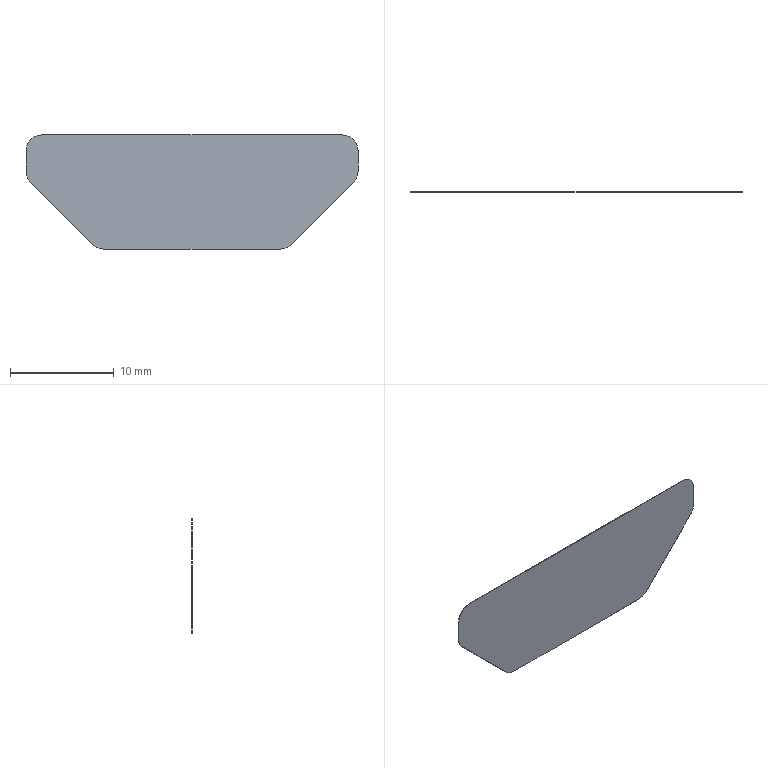Part | NX | features BREP 1 | 1 solid | 14 faces | box 32 x 0.05 x 11 mm | volume 15.176 mm3 | plane 8 | cylinder 6 | commonest cylinder face diameters 3 x6
STEP:
#1=CARTESIAN_POINT('',(0.,0.,7.5));
#2=VERTEX_POINT('',#1);
#3=CARTESIAN_POINT('',(0.,0.05,7.5));
#4=VERTEX_POINT('',#3);
#5=CARTESIAN_POINT('',(0.,0.,7.5));
#6=DIRECTION('',(0.,1.,0.));
#7=VECTOR('',#6,1000.);
#8=LINE('',#5,#7);
#9=EDGE_CURVE('',#2,#4,#8,.T.);
#10=ORIENTED_EDGE('',*,*,#9,.F.);
#11=CARTESIAN_POINT('',(0.,0.,9.5));
#12=VERTEX_POINT('',#11);
#13=CARTESIAN_POINT('',(0.,0.,7.5));
#14=DIRECTION('',(0.,0.,1.));
#15=VECTOR('',#14,1000.);
#16=LINE('',#13,#15);
#17=EDGE_CURVE('',#2,#12,#16,.T.);
#18=ORIENTED_EDGE('',*,*,#17,.T.);
#19=CARTESIAN_POINT('',(0.,0.05,9.5));
#20=VERTEX_POINT('',#19);
#21=CARTESIAN_POINT('',(0.,0.,9.5));
#22=DIRECTION('',(0.,1.,0.));
#23=VECTOR('',#22,1000.);
#24=LINE('',#21,#23);
#25=EDGE_CURVE('',#12,#20,#24,.T.);
#26=ORIENTED_EDGE('',*,*,#25,.T.);
#27=CARTESIAN_POINT('',(0.,0.05,7.5));
#28=DIRECTION('',(0.,0.,1.));
#29=VECTOR('',#28,1000.);
#30=LINE('',#27,#29);
#31=EDGE_CURVE('',#4,#20,#30,.T.);
#32=ORIENTED_EDGE('',*,*,#31,.F.);
#33=EDGE_LOOP('',(#10,#18,#26,#32));
#34=FACE_BOUND('',#33,.T.);
#35=CARTESIAN_POINT('',(0.,0.,7.5));
#36=DIRECTION('',(-1.,0.,0.));
#37=DIRECTION('',(0.,0.,-1.));
#38=AXIS2_PLACEMENT_3D('',#35,#36,#37);
#39=PLANE('',#38);
#40=ADVANCED_FACE('',(#34),#39,.T.);
#41=ORIENTED_EDGE('',*,*,#25,.F.);
#42=CARTESIAN_POINT('',(1.5,0.,11.));
#43=VERTEX_POINT('',#42);
#44=CARTESIAN_POINT('',(1.5,0.,9.5));
#45=DIRECTION('',(0.,1.,0.));
#46=DIRECTION('',(-1.,0.,0.));
#47=AXIS2_PLACEMENT_3D('',#44,#45,#46);
#48=CIRCLE('',#47,1.5);
#49=EDGE_CURVE('',#12,#43,#48,.T.);
#50=ORIENTED_EDGE('',*,*,#49,.T.);
#51=CARTESIAN_POINT('',(1.5,0.05,11.));
#52=VERTEX_POINT('',#51);
#53=CARTESIAN_POINT('',(1.5,0.,11.));
#54=DIRECTION('',(0.,1.,0.));
#55=VECTOR('',#54,1000.);
#56=LINE('',#53,#55);
#57=EDGE_CURVE('',#43,#52,#56,.T.);
#58=ORIENTED_EDGE('',*,*,#57,.T.);
#59=CARTESIAN_POINT('',(1.5,0.05,9.5));
#60=DIRECTION('',(0.,1.,0.));
#61=DIRECTION('',(-1.,0.,0.));
#62=AXIS2_PLACEMENT_3D('',#59,#60,#61);
#63=CIRCLE('',#62,1.5);
#64=EDGE_CURVE('',#20,#52,#63,.T.);
#65=ORIENTED_EDGE('',*,*,#64,.F.);
#66=EDGE_LOOP('',(#41,#50,#58,#65));
#67=FACE_BOUND('',#66,.T.);
#68=CARTESIAN_POINT('',(1.5,0.,9.5));
#69=DIRECTION('',(0.,1.,0.));
#70=DIRECTION('',(-0.7071,0.,0.7071));
#71=AXIS2_PLACEMENT_3D('',#68,#69,#70);
#72=CYLINDRICAL_SURFACE('',#71,1.5);
#73=ADVANCED_FACE('',(#67),#72,.T.);
#74=ORIENTED_EDGE('',*,*,#57,.F.);
#75=CARTESIAN_POINT('',(30.5,0.,11.));
#76=VERTEX_POINT('',#75);
#77=CARTESIAN_POINT('',(1.5,0.,11.));
#78=DIRECTION('',(1.,0.,0.));
#79=VECTOR('',#78,1000.);
#80=LINE('',#77,#79);
#81=EDGE_CURVE('',#43,#76,#80,.T.);
#82=ORIENTED_EDGE('',*,*,#81,.T.);
#83=CARTESIAN_POINT('',(30.5,0.05,11.));
#84=VERTEX_POINT('',#83);
#85=CARTESIAN_POINT('',(30.5,0.,11.));
#86=DIRECTION('',(0.,1.,0.));
#87=VECTOR('',#86,1000.);
#88=LINE('',#85,#87);
#89=EDGE_CURVE('',#76,#84,#88,.T.);
#90=ORIENTED_EDGE('',*,*,#89,.T.);
#91=CARTESIAN_POINT('',(1.5,0.05,11.));
#92=DIRECTION('',(1.,0.,0.));
#93=VECTOR('',#92,1000.);
#94=LINE('',#91,#93);
#95=EDGE_CURVE('',#52,#84,#94,.T.);
#96=ORIENTED_EDGE('',*,*,#95,.F.);
#97=EDGE_LOOP('',(#74,#82,#90,#96));
#98=FACE_BOUND('',#97,.T.);
#99=CARTESIAN_POINT('',(1.5,0.,11.));
#100=DIRECTION('',(0.,0.,1.));
#101=DIRECTION('',(-1.,0.,0.));
#102=AXIS2_PLACEMENT_3D('',#99,#100,#101);
#103=PLANE('',#102);
#104=ADVANCED_FACE('',(#98),#103,.T.);
#105=ORIENTED_EDGE('',*,*,#89,.F.);
#106=CARTESIAN_POINT('',(32.,0.,9.5));
#107=VERTEX_POINT('',#106);
#108=CARTESIAN_POINT('',(30.5,0.,9.5));
#109=DIRECTION('',(0.,1.,0.));
#110=DIRECTION('',(0.,0.,1.));
#111=AXIS2_PLACEMENT_3D('',#108,#109,#110);
#112=CIRCLE('',#111,1.5);
#113=EDGE_CURVE('',#76,#107,#112,.T.);
#114=ORIENTED_EDGE('',*,*,#113,.T.);
#115=CARTESIAN_POINT('',(32.,0.05,9.5));
#116=VERTEX_POINT('',#115);
#117=CARTESIAN_POINT('',(32.,0.,9.5));
#118=DIRECTION('',(0.,1.,0.));
#119=VECTOR('',#118,1000.);
#120=LINE('',#117,#119);
#121=EDGE_CURVE('',#107,#116,#120,.T.);
#122=ORIENTED_EDGE('',*,*,#121,.T.);
#123=CARTESIAN_POINT('',(30.5,0.05,9.5));
#124=DIRECTION('',(0.,1.,0.));
#125=DIRECTION('',(0.,0.,1.));
#126=AXIS2_PLACEMENT_3D('',#123,#124,#125);
#127=CIRCLE('',#126,1.5);
#128=EDGE_CURVE('',#84,#116,#127,.T.);
#129=ORIENTED_EDGE('',*,*,#128,.F.);
#130=EDGE_LOOP('',(#105,#114,#122,#129));
#131=FACE_BOUND('',#130,.T.);
#132=CARTESIAN_POINT('',(30.5,0.,9.5));
#133=DIRECTION('',(0.,1.,0.));
#134=DIRECTION('',(0.7071,0.,0.7071));
#135=AXIS2_PLACEMENT_3D('',#132,#133,#134);
#136=CYLINDRICAL_SURFACE('',#135,1.5);
#137=ADVANCED_FACE('',(#131),#136,.T.);
#138=ORIENTED_EDGE('',*,*,#121,.F.);
#139=CARTESIAN_POINT('',(32.,0.,7.5));
#140=VERTEX_POINT('',#139);
#141=CARTESIAN_POINT('',(32.,0.,9.5));
#142=DIRECTION('',(0.,0.,-1.));
#143=VECTOR('',#142,1000.);
#144=LINE('',#141,#143);
#145=EDGE_CURVE('',#107,#140,#144,.T.);
#146=ORIENTED_EDGE('',*,*,#145,.T.);
#147=CARTESIAN_POINT('',(32.,0.05,7.5));
#148=VERTEX_POINT('',#147);
#149=CARTESIAN_POINT('',(32.,0.,7.5));
#150=DIRECTION('',(0.,1.,0.));
#151=VECTOR('',#150,1000.);
#152=LINE('',#149,#151);
#153=EDGE_CURVE('',#140,#148,#152,.T.);
#154=ORIENTED_EDGE('',*,*,#153,.T.);
#155=CARTESIAN_POINT('',(32.,0.05,9.5));
#156=DIRECTION('',(0.,0.,-1.));
#157=VECTOR('',#156,1000.);
#158=LINE('',#155,#157);
#159=EDGE_CURVE('',#116,#148,#158,.T.);
#160=ORIENTED_EDGE('',*,*,#159,.F.);
#161=EDGE_LOOP('',(#138,#146,#154,#160));
#162=FACE_BOUND('',#161,.T.);
#163=CARTESIAN_POINT('',(32.,0.,9.5));
#164=DIRECTION('',(1.,0.,0.));
#165=DIRECTION('',(0.,-1.,0.));
#166=AXIS2_PLACEMENT_3D('',#163,#164,#165);
#167=PLANE('',#166);
#168=ADVANCED_FACE('',(#162),#167,.T.);
#169=ORIENTED_EDGE('',*,*,#153,.F.);
#170=CARTESIAN_POINT('',(31.561,0.,6.439));
#171=VERTEX_POINT('',#170);
#172=CARTESIAN_POINT('',(30.5,0.,7.5));
#173=DIRECTION('',(0.,1.,0.));
#174=DIRECTION('',(1.,0.,0.));
#175=AXIS2_PLACEMENT_3D('',#172,#173,#174);
#176=CIRCLE('',#175,1.5);
#177=EDGE_CURVE('',#140,#171,#176,.T.);
#178=ORIENTED_EDGE('',*,*,#177,.T.);
#179=CARTESIAN_POINT('',(31.561,0.05,6.439));
#180=VERTEX_POINT('',#179);
#181=CARTESIAN_POINT('',(31.561,0.,6.439));
#182=DIRECTION('',(0.,1.,0.));
#183=VECTOR('',#182,1000.);
#184=LINE('',#181,#183);
#185=EDGE_CURVE('',#171,#180,#184,.T.);
#186=ORIENTED_EDGE('',*,*,#185,.T.);
#187=CARTESIAN_POINT('',(30.5,0.05,7.5));
#188=DIRECTION('',(0.,1.,0.));
#189=DIRECTION('',(1.,0.,0.));
#190=AXIS2_PLACEMENT_3D('',#187,#188,#189);
#191=CIRCLE('',#190,1.5);
#192=EDGE_CURVE('',#148,#180,#191,.T.);
#193=ORIENTED_EDGE('',*,*,#192,.F.);
#194=EDGE_LOOP('',(#169,#178,#186,#193));
#195=FACE_BOUND('',#194,.T.);
#196=CARTESIAN_POINT('',(30.5,0.,7.5));
#197=DIRECTION('',(0.,1.,0.));
#198=DIRECTION('',(0.9239,0.,-0.3827));
#199=AXIS2_PLACEMENT_3D('',#196,#197,#198);
#200=CYLINDRICAL_SURFACE('',#199,1.5);
#201=ADVANCED_FACE('',(#195),#200,.T.);
#202=ORIENTED_EDGE('',*,*,#185,.F.);
#203=CARTESIAN_POINT('',(25.561,0.,0.4393));
#204=VERTEX_POINT('',#203);
#205=CARTESIAN_POINT('',(31.561,0.,6.439));
#206=DIRECTION('',(-0.7071,0.,-0.7071));
#207=VECTOR('',#206,1000.);
#208=LINE('',#205,#207);
#209=EDGE_CURVE('',#171,#204,#208,.T.);
#210=ORIENTED_EDGE('',*,*,#209,.T.);
#211=CARTESIAN_POINT('',(25.561,0.05,0.4393));
#212=VERTEX_POINT('',#211);
#213=CARTESIAN_POINT('',(25.561,0.,0.4393));
#214=DIRECTION('',(0.,1.,0.));
#215=VECTOR('',#214,1000.);
#216=LINE('',#213,#215);
#217=EDGE_CURVE('',#204,#212,#216,.T.);
#218=ORIENTED_EDGE('',*,*,#217,.T.);
#219=CARTESIAN_POINT('',(31.561,0.05,6.439));
#220=DIRECTION('',(-0.7071,0.,-0.7071));
#221=VECTOR('',#220,1000.);
#222=LINE('',#219,#221);
#223=EDGE_CURVE('',#180,#212,#222,.T.);
#224=ORIENTED_EDGE('',*,*,#223,.F.);
#225=EDGE_LOOP('',(#202,#210,#218,#224));
#226=FACE_BOUND('',#225,.T.);
#227=CARTESIAN_POINT('',(31.561,0.,6.439));
#228=DIRECTION('',(0.7071,0.,-0.7071));
#229=DIRECTION('',(0.,1.,0.));
#230=AXIS2_PLACEMENT_3D('',#227,#228,#229);
#231=PLANE('',#230);
#232=ADVANCED_FACE('',(#226),#231,.T.);
#233=ORIENTED_EDGE('',*,*,#217,.F.);
#234=CARTESIAN_POINT('',(24.5,0.,0.));
#235=VERTEX_POINT('',#234);
#236=CARTESIAN_POINT('',(24.5,0.,1.5));
#237=DIRECTION('',(0.,1.,0.));
#238=DIRECTION('',(0.7071,0.,-0.7071));
#239=AXIS2_PLACEMENT_3D('',#236,#237,#238);
#240=CIRCLE('',#239,1.5);
#241=EDGE_CURVE('',#204,#235,#240,.T.);
#242=ORIENTED_EDGE('',*,*,#241,.T.);
#243=CARTESIAN_POINT('',(24.5,0.05,0.));
#244=VERTEX_POINT('',#243);
#245=CARTESIAN_POINT('',(24.5,0.,0.));
#246=DIRECTION('',(0.,1.,0.));
#247=VECTOR('',#246,1000.);
#248=LINE('',#245,#247);
#249=EDGE_CURVE('',#235,#244,#248,.T.);
#250=ORIENTED_EDGE('',*,*,#249,.T.);
#251=CARTESIAN_POINT('',(24.5,0.05,1.5));
#252=DIRECTION('',(0.,1.,0.));
#253=DIRECTION('',(0.7071,0.,-0.7071));
#254=AXIS2_PLACEMENT_3D('',#251,#252,#253);
#255=CIRCLE('',#254,1.5);
#256=EDGE_CURVE('',#212,#244,#255,.T.);
#257=ORIENTED_EDGE('',*,*,#256,.F.);
#258=EDGE_LOOP('',(#233,#242,#250,#257));
#259=FACE_BOUND('',#258,.T.);
#260=CARTESIAN_POINT('',(24.5,0.,1.5));
#261=DIRECTION('',(0.,1.,0.));
#262=DIRECTION('',(0.3827,0.,-0.9239));
#263=AXIS2_PLACEMENT_3D('',#260,#261,#262);
#264=CYLINDRICAL_SURFACE('',#263,1.5);
#265=ADVANCED_FACE('',(#259),#264,.T.);
#266=ORIENTED_EDGE('',*,*,#249,.F.);
#267=CARTESIAN_POINT('',(7.5,0.,0.));
#268=VERTEX_POINT('',#267);
#269=CARTESIAN_POINT('',(24.5,0.,0.));
#270=DIRECTION('',(-1.,0.,0.));
#271=VECTOR('',#270,1000.);
#272=LINE('',#269,#271);
#273=EDGE_CURVE('',#235,#268,#272,.T.);
#274=ORIENTED_EDGE('',*,*,#273,.T.);
#275=CARTESIAN_POINT('',(7.5,0.05,0.));
#276=VERTEX_POINT('',#275);
#277=CARTESIAN_POINT('',(7.5,0.,0.));
#278=DIRECTION('',(0.,1.,0.));
#279=VECTOR('',#278,1000.);
#280=LINE('',#277,#279);
#281=EDGE_CURVE('',#268,#276,#280,.T.);
#282=ORIENTED_EDGE('',*,*,#281,.T.);
#283=CARTESIAN_POINT('',(24.5,0.05,0.));
#284=DIRECTION('',(-1.,0.,0.));
#285=VECTOR('',#284,1000.);
#286=LINE('',#283,#285);
#287=EDGE_CURVE('',#244,#276,#286,.T.);
#288=ORIENTED_EDGE('',*,*,#287,.F.);
#289=EDGE_LOOP('',(#266,#274,#282,#288));
#290=FACE_BOUND('',#289,.T.);
#291=CARTESIAN_POINT('',(24.5,0.,0.));
#292=DIRECTION('',(0.,0.,-1.));
#293=DIRECTION('',(0.,1.,0.));
#294=AXIS2_PLACEMENT_3D('',#291,#292,#293);
#295=PLANE('',#294);
#296=ADVANCED_FACE('',(#290),#295,.T.);
#297=ORIENTED_EDGE('',*,*,#281,.F.);
#298=CARTESIAN_POINT('',(6.439,0.,0.4393));
#299=VERTEX_POINT('',#298);
#300=CARTESIAN_POINT('',(7.5,0.,1.5));
#301=DIRECTION('',(0.,1.,0.));
#302=DIRECTION('',(0.,0.,-1.));
#303=AXIS2_PLACEMENT_3D('',#300,#301,#302);
#304=CIRCLE('',#303,1.5);
#305=EDGE_CURVE('',#268,#299,#304,.T.);
#306=ORIENTED_EDGE('',*,*,#305,.T.);
#307=CARTESIAN_POINT('',(6.439,0.05,0.4393));
#308=VERTEX_POINT('',#307);
#309=CARTESIAN_POINT('',(6.439,0.,0.4393));
#310=DIRECTION('',(0.,1.,0.));
#311=VECTOR('',#310,1000.);
#312=LINE('',#309,#311);
#313=EDGE_CURVE('',#299,#308,#312,.T.);
#314=ORIENTED_EDGE('',*,*,#313,.T.);
#315=CARTESIAN_POINT('',(7.5,0.05,1.5));
#316=DIRECTION('',(0.,1.,0.));
#317=DIRECTION('',(0.,0.,-1.));
#318=AXIS2_PLACEMENT_3D('',#315,#316,#317);
#319=CIRCLE('',#318,1.5);
#320=EDGE_CURVE('',#276,#308,#319,.T.);
#321=ORIENTED_EDGE('',*,*,#320,.F.);
#322=EDGE_LOOP('',(#297,#306,#314,#321));
#323=FACE_BOUND('',#322,.T.);
#324=CARTESIAN_POINT('',(7.5,0.,1.5));
#325=DIRECTION('',(0.,1.,0.));
#326=DIRECTION('',(-0.3827,0.,-0.9239));
#327=AXIS2_PLACEMENT_3D('',#324,#325,#326);
#328=CYLINDRICAL_SURFACE('',#327,1.5);
#329=ADVANCED_FACE('',(#323),#328,.T.);
#330=ORIENTED_EDGE('',*,*,#313,.F.);
#331=CARTESIAN_POINT('',(0.4393,0.,6.439));
#332=VERTEX_POINT('',#331);
#333=CARTESIAN_POINT('',(6.439,0.,0.4393));
#334=DIRECTION('',(-0.7071,0.,0.7071));
#335=VECTOR('',#334,1000.);
#336=LINE('',#333,#335);
#337=EDGE_CURVE('',#299,#332,#336,.T.);
#338=ORIENTED_EDGE('',*,*,#337,.T.);
#339=CARTESIAN_POINT('',(0.4393,0.05,6.439));
#340=VERTEX_POINT('',#339);
#341=CARTESIAN_POINT('',(0.4393,0.,6.439));
#342=DIRECTION('',(0.,1.,0.));
#343=VECTOR('',#342,1000.);
#344=LINE('',#341,#343);
#345=EDGE_CURVE('',#332,#340,#344,.T.);
#346=ORIENTED_EDGE('',*,*,#345,.T.);
#347=CARTESIAN_POINT('',(6.439,0.05,0.4393));
#348=DIRECTION('',(-0.7071,0.,0.7071));
#349=VECTOR('',#348,1000.);
#350=LINE('',#347,#349);
#351=EDGE_CURVE('',#308,#340,#350,.T.);
#352=ORIENTED_EDGE('',*,*,#351,.F.);
#353=EDGE_LOOP('',(#330,#338,#346,#352));
#354=FACE_BOUND('',#353,.T.);
#355=CARTESIAN_POINT('',(6.439,0.,0.4393));
#356=DIRECTION('',(-0.7071,0.,-0.7071));
#357=DIRECTION('',(0.7071,0.,-0.7071));
#358=AXIS2_PLACEMENT_3D('',#355,#356,#357);
#359=PLANE('',#358);
#360=ADVANCED_FACE('',(#354),#359,.T.);
#361=ORIENTED_EDGE('',*,*,#345,.F.);
#362=CARTESIAN_POINT('',(1.5,0.,7.5));
#363=DIRECTION('',(0.,1.,0.));
#364=DIRECTION('',(-0.7071,0.,-0.7071));
#365=AXIS2_PLACEMENT_3D('',#362,#363,#364);
#366=CIRCLE('',#365,1.5);
#367=EDGE_CURVE('',#332,#2,#366,.T.);
#368=ORIENTED_EDGE('',*,*,#367,.T.);
#369=ORIENTED_EDGE('',*,*,#9,.T.);
#370=CARTESIAN_POINT('',(1.5,0.05,7.5));
#371=DIRECTION('',(0.,1.,0.));
#372=DIRECTION('',(-0.7071,0.,-0.7071));
#373=AXIS2_PLACEMENT_3D('',#370,#371,#372);
#374=CIRCLE('',#373,1.5);
#375=EDGE_CURVE('',#340,#4,#374,.T.);
#376=ORIENTED_EDGE('',*,*,#375,.F.);
#377=EDGE_LOOP('',(#361,#368,#369,#376));
#378=FACE_BOUND('',#377,.T.);
#379=CARTESIAN_POINT('',(1.5,0.,7.5));
#380=DIRECTION('',(0.,1.,0.));
#381=DIRECTION('',(-0.9239,0.,-0.3827));
#382=AXIS2_PLACEMENT_3D('',#379,#380,#381);
#383=CYLINDRICAL_SURFACE('',#382,1.5);
#384=ADVANCED_FACE('',(#378),#383,.T.);
#385=ORIENTED_EDGE('',*,*,#17,.F.);
#386=ORIENTED_EDGE('',*,*,#367,.F.);
#387=ORIENTED_EDGE('',*,*,#337,.F.);
#388=ORIENTED_EDGE('',*,*,#305,.F.);
#389=ORIENTED_EDGE('',*,*,#273,.F.);
#390=ORIENTED_EDGE('',*,*,#241,.F.);
#391=ORIENTED_EDGE('',*,*,#209,.F.);
#392=ORIENTED_EDGE('',*,*,#177,.F.);
#393=ORIENTED_EDGE('',*,*,#145,.F.);
#394=ORIENTED_EDGE('',*,*,#113,.F.);
#395=ORIENTED_EDGE('',*,*,#81,.F.);
#396=ORIENTED_EDGE('',*,*,#49,.F.);
#397=EDGE_LOOP('',(#385,#386,#387,#388,#389,#390,#391,#392,#393,#394,#395,#396));
#398=FACE_BOUND('',#397,.T.);
#399=CARTESIAN_POINT('',(32.,0.,0.));
#400=DIRECTION('',(0.,-1.,0.));
#401=DIRECTION('',(0.,0.,1.));
#402=AXIS2_PLACEMENT_3D('',#399,#400,#401);
#403=PLANE('',#402);
#404=ADVANCED_FACE('',(#398),#403,.T.);
#405=ORIENTED_EDGE('',*,*,#31,.T.);
#406=ORIENTED_EDGE('',*,*,#64,.T.);
#407=ORIENTED_EDGE('',*,*,#95,.T.);
#408=ORIENTED_EDGE('',*,*,#128,.T.);
#409=ORIENTED_EDGE('',*,*,#159,.T.);
#410=ORIENTED_EDGE('',*,*,#192,.T.);
#411=ORIENTED_EDGE('',*,*,#223,.T.);
#412=ORIENTED_EDGE('',*,*,#256,.T.);
#413=ORIENTED_EDGE('',*,*,#287,.T.);
#414=ORIENTED_EDGE('',*,*,#320,.T.);
#415=ORIENTED_EDGE('',*,*,#351,.T.);
#416=ORIENTED_EDGE('',*,*,#375,.T.);
#417=EDGE_LOOP('',(#405,#406,#407,#408,#409,#410,#411,#412,#413,#414,#415,#416));
#418=FACE_BOUND('',#417,.T.);
#419=CARTESIAN_POINT('',(32.,0.05,0.));
#420=DIRECTION('',(0.,1.,0.));
#421=DIRECTION('',(-1.,0.,0.));
#422=AXIS2_PLACEMENT_3D('',#419,#420,#421);
#423=PLANE('',#422);
#424=ADVANCED_FACE('',(#418),#423,.T.);
#425=CLOSED_SHELL('',(#40,#73,#104,#137,#168,#201,#232,#265,#296,#329,#360,#384,#404,#424));
#426=MANIFOLD_SOLID_BREP('',#425);
#427=(LENGTH_UNIT()NAMED_UNIT(*)SI_UNIT(.MILLI.,.METRE.));
#428=UNCERTAINTY_MEASURE_WITH_UNIT(LENGTH_MEASURE(0.00001),#427,'','');
#429=(NAMED_UNIT(*)PLANE_ANGLE_UNIT()SI_UNIT($,.RADIAN.));
#430=(NAMED_UNIT(*)SI_UNIT($,.STERADIAN.)SOLID_ANGLE_UNIT());
#431=(GEOMETRIC_REPRESENTATION_CONTEXT(3)GLOBAL_UNCERTAINTY_ASSIGNED_CONTEXT((#428))GLOBAL_UNIT_ASSIGNED_CONTEXT((#427,#429,#430))REPRESENTATION_CONTEXT('',''));
#432=ADVANCED_BREP_SHAPE_REPRESENTATION('',(#426),#431);